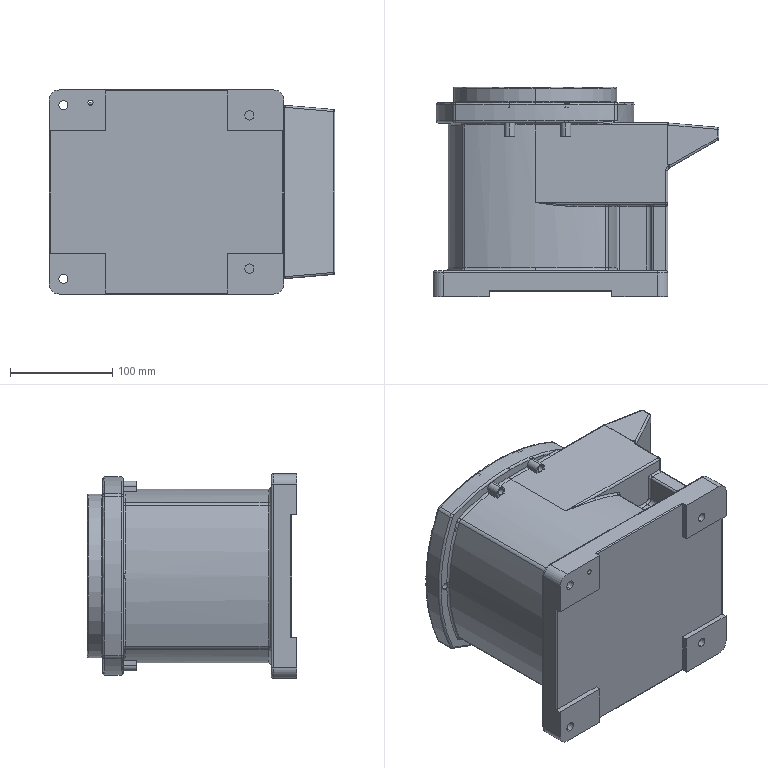Part | SolidWorks | features ICE 12, Fillet 7, 3DProfileFeature 2, Chamfer 2, HoleWzd 2, MirrorPattern 2, Extrusion 1 | 1 solid | 314 faces | box 280 x 205 x 200 mm | volume 6648707 mm3 | cylinder 138 | torus 77 | plane 68 | spline 13 | cone 10 | sphere 8 | commonest cylinder face diameters 4 x38 7 x20 13 x20 10 x17 9 x8 15 x8